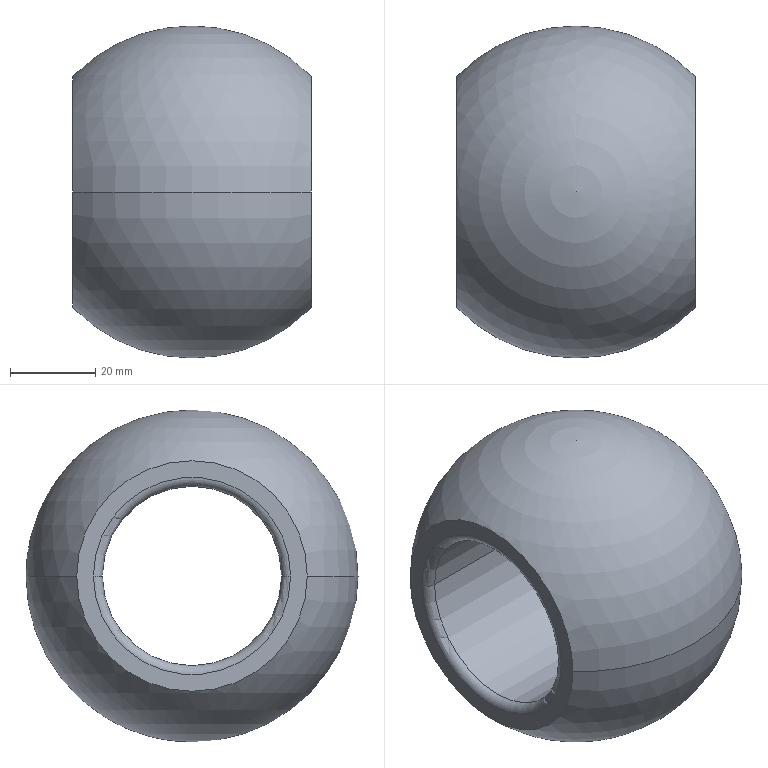Part | STEP file | Rod end bearing 1 | 1 solid | 10 faces | box 56 x 77.805 x 77.805 mm | volume 142436 mm3 | torus 4 | sphere 2 | cylinder 2 | plane 2 | commonest cylinder face diameters 42 x2
STEP:
#1=CARTESIAN_POINT('',(28.,27.007,261.));
#2=VERTEX_POINT('',#1);
#3=CARTESIAN_POINT('',(28.,-27.007,261.));
#4=VERTEX_POINT('',#3);
#5=CARTESIAN_POINT('',(28.,0.,261.));
#6=DIRECTION('',(-1.,0.,0.));
#7=DIRECTION('',(0.,-1.,0.));
#8=AXIS2_PLACEMENT_3D('',#5,#6,#7);
#9=CIRCLE('',#8,27.007);
#10=EDGE_CURVE('',#2,#4,#9,.T.);
#11=ORIENTED_EDGE('',*,*,#10,.T.);
#12=CARTESIAN_POINT('',(-28.,-27.007,261.));
#13=VERTEX_POINT('',#12);
#14=CARTESIAN_POINT('',(0.,0.,261.));
#15=DIRECTION('',(0.,0.,-1.));
#16=DIRECTION('',(0.,1.,0.));
#17=AXIS2_PLACEMENT_3D('',#14,#15,#16);
#18=CIRCLE('',#17,38.902);
#19=EDGE_CURVE('',#4,#13,#18,.T.);
#20=ORIENTED_EDGE('',*,*,#19,.T.);
#21=CARTESIAN_POINT('',(-28.,27.007,261.));
#22=VERTEX_POINT('',#21);
#23=CARTESIAN_POINT('',(-28.,0.,261.));
#24=DIRECTION('',(-1.,0.,0.));
#25=DIRECTION('',(0.,-1.,0.));
#26=AXIS2_PLACEMENT_3D('',#23,#24,#25);
#27=CIRCLE('',#26,27.007);
#28=EDGE_CURVE('',#22,#13,#27,.T.);
#29=ORIENTED_EDGE('',*,*,#28,.F.);
#30=CARTESIAN_POINT('',(0.,0.,261.));
#31=DIRECTION('',(0.,0.,1.));
#32=DIRECTION('',(1.,0.,0.));
#33=AXIS2_PLACEMENT_3D('',#30,#31,#32);
#34=CIRCLE('',#33,38.902);
#35=EDGE_CURVE('',#2,#22,#34,.T.);
#36=ORIENTED_EDGE('',*,*,#35,.F.);
#37=EDGE_LOOP('',(#11,#20,#29,#36));
#38=FACE_OUTER_BOUND('',#37,.T.);
#39=CARTESIAN_POINT('',(0.,0.,261.));
#40=DIRECTION('',(0.,0.,-1.));
#41=DIRECTION('',(0.,1.,0.));
#42=AXIS2_PLACEMENT_3D('',#39,#40,#41);
#43=SPHERICAL_SURFACE('',#42,38.902);
#44=ADVANCED_FACE('',(#38),#43,.T.);
#45=CARTESIAN_POINT('',(-28.,-23.1,261.));
#46=VERTEX_POINT('',#45);
#47=CARTESIAN_POINT('',(-28.,23.1,261.));
#48=VERTEX_POINT('',#47);
#49=CARTESIAN_POINT('',(-28.,0.,261.));
#50=DIRECTION('',(-1.,0.,0.));
#51=DIRECTION('',(0.,-1.,0.));
#52=AXIS2_PLACEMENT_3D('',#49,#50,#51);
#53=CIRCLE('',#52,23.1);
#54=EDGE_CURVE('',#46,#48,#53,.T.);
#55=ORIENTED_EDGE('',*,*,#54,.T.);
#56=CARTESIAN_POINT('',(-25.9,21.,261.));
#57=VERTEX_POINT('',#56);
#58=CARTESIAN_POINT('',(-25.9,23.1,261.));
#59=DIRECTION('',(0.,0.,1.));
#60=DIRECTION('',(0.,-1.,0.));
#61=AXIS2_PLACEMENT_3D('',#58,#59,#60);
#62=CIRCLE('',#61,2.1);
#63=EDGE_CURVE('',#48,#57,#62,.T.);
#64=ORIENTED_EDGE('',*,*,#63,.T.);
#65=CARTESIAN_POINT('',(-25.9,-21.,261.));
#66=VERTEX_POINT('',#65);
#67=CARTESIAN_POINT('',(-25.9,0.,261.));
#68=DIRECTION('',(-1.,0.,0.));
#69=DIRECTION('',(0.,-1.,0.));
#70=AXIS2_PLACEMENT_3D('',#67,#68,#69);
#71=CIRCLE('',#70,21.);
#72=EDGE_CURVE('',#66,#57,#71,.T.);
#73=ORIENTED_EDGE('',*,*,#72,.F.);
#74=CARTESIAN_POINT('',(-25.9,-23.1,261.));
#75=DIRECTION('',(0.,0.,-1.));
#76=DIRECTION('',(-1.,0.,0.));
#77=AXIS2_PLACEMENT_3D('',#74,#75,#76);
#78=CIRCLE('',#77,2.1);
#79=EDGE_CURVE('',#46,#66,#78,.T.);
#80=ORIENTED_EDGE('',*,*,#79,.F.);
#81=EDGE_LOOP('',(#55,#64,#73,#80));
#82=FACE_OUTER_BOUND('',#81,.T.);
#83=CARTESIAN_POINT('',(-25.9,0.,261.));
#84=DIRECTION('',(-1.,0.,0.));
#85=DIRECTION('',(0.,-1.,0.));
#86=AXIS2_PLACEMENT_3D('',#83,#84,#85);
#87=TOROIDAL_SURFACE('',#86,23.1,2.1);
#88=ADVANCED_FACE('',(#82),#87,.T.);
#89=CARTESIAN_POINT('',(25.9,21.,261.));
#90=VERTEX_POINT('',#89);
#91=CARTESIAN_POINT('',(25.9,-21.,261.));
#92=VERTEX_POINT('',#91);
#93=CARTESIAN_POINT('',(25.9,0.,261.));
#94=DIRECTION('',(-1.,0.,0.));
#95=DIRECTION('',(0.,-1.,0.));
#96=AXIS2_PLACEMENT_3D('',#93,#94,#95);
#97=CIRCLE('',#96,21.);
#98=EDGE_CURVE('',#90,#92,#97,.T.);
#99=ORIENTED_EDGE('',*,*,#98,.F.);
#100=CARTESIAN_POINT('',(28.,21.,261.));
#101=DIRECTION('',(-1.,0.,0.));
#102=VECTOR('',#101,1000.);
#103=LINE('',#100,#102);
#104=EDGE_CURVE('',#90,#57,#103,.T.);
#105=ORIENTED_EDGE('',*,*,#104,.T.);
#106=CARTESIAN_POINT('',(-25.9,0.,261.));
#107=DIRECTION('',(-1.,0.,0.));
#108=DIRECTION('',(0.,-1.,0.));
#109=AXIS2_PLACEMENT_3D('',#106,#107,#108);
#110=CIRCLE('',#109,21.);
#111=EDGE_CURVE('',#57,#66,#110,.T.);
#112=ORIENTED_EDGE('',*,*,#111,.T.);
#113=CARTESIAN_POINT('',(28.,-21.,261.));
#114=DIRECTION('',(-1.,0.,0.));
#115=VECTOR('',#114,1000.);
#116=LINE('',#113,#115);
#117=EDGE_CURVE('',#92,#66,#116,.T.);
#118=ORIENTED_EDGE('',*,*,#117,.F.);
#119=EDGE_LOOP('',(#99,#105,#112,#118));
#120=FACE_OUTER_BOUND('',#119,.T.);
#121=CARTESIAN_POINT('',(28.,0.,261.));
#122=DIRECTION('',(-1.,0.,0.));
#123=DIRECTION('',(0.,-1.,0.));
#124=AXIS2_PLACEMENT_3D('',#121,#122,#123);
#125=CYLINDRICAL_SURFACE('',#124,21.);
#126=ADVANCED_FACE('',(#120),#125,.F.);
#127=CARTESIAN_POINT('',(25.9,0.,261.));
#128=DIRECTION('',(-1.,0.,0.));
#129=DIRECTION('',(0.,-1.,0.));
#130=AXIS2_PLACEMENT_3D('',#127,#128,#129);
#131=CIRCLE('',#130,21.);
#132=EDGE_CURVE('',#92,#90,#131,.T.);
#133=ORIENTED_EDGE('',*,*,#132,.T.);
#134=CARTESIAN_POINT('',(28.,23.1,261.));
#135=VERTEX_POINT('',#134);
#136=CARTESIAN_POINT('',(25.9,23.1,261.));
#137=DIRECTION('',(0.,0.,1.));
#138=DIRECTION('',(0.,-1.,0.));
#139=AXIS2_PLACEMENT_3D('',#136,#137,#138);
#140=CIRCLE('',#139,2.1);
#141=EDGE_CURVE('',#90,#135,#140,.T.);
#142=ORIENTED_EDGE('',*,*,#141,.T.);
#143=CARTESIAN_POINT('',(28.,-23.1,261.));
#144=VERTEX_POINT('',#143);
#145=CARTESIAN_POINT('',(28.,0.,261.));
#146=DIRECTION('',(-1.,0.,0.));
#147=DIRECTION('',(0.,-1.,0.));
#148=AXIS2_PLACEMENT_3D('',#145,#146,#147);
#149=CIRCLE('',#148,23.1);
#150=EDGE_CURVE('',#144,#135,#149,.T.);
#151=ORIENTED_EDGE('',*,*,#150,.F.);
#152=CARTESIAN_POINT('',(25.9,-23.1,261.));
#153=DIRECTION('',(0.,0.,-1.));
#154=DIRECTION('',(-1.,0.,0.));
#155=AXIS2_PLACEMENT_3D('',#152,#153,#154);
#156=CIRCLE('',#155,2.1);
#157=EDGE_CURVE('',#92,#144,#156,.T.);
#158=ORIENTED_EDGE('',*,*,#157,.F.);
#159=EDGE_LOOP('',(#133,#142,#151,#158));
#160=FACE_OUTER_BOUND('',#159,.T.);
#161=CARTESIAN_POINT('',(25.9,0.,261.));
#162=DIRECTION('',(-1.,0.,0.));
#163=DIRECTION('',(0.,-1.,0.));
#164=AXIS2_PLACEMENT_3D('',#161,#162,#163);
#165=TOROIDAL_SURFACE('',#164,23.1,2.1);
#166=ADVANCED_FACE('',(#160),#165,.T.);
#167=ORIENTED_EDGE('',*,*,#141,.F.);
#168=ORIENTED_EDGE('',*,*,#98,.T.);
#169=ORIENTED_EDGE('',*,*,#157,.T.);
#170=CARTESIAN_POINT('',(28.,0.,261.));
#171=DIRECTION('',(-1.,0.,0.));
#172=DIRECTION('',(0.,-1.,0.));
#173=AXIS2_PLACEMENT_3D('',#170,#171,#172);
#174=CIRCLE('',#173,23.1);
#175=EDGE_CURVE('',#135,#144,#174,.T.);
#176=ORIENTED_EDGE('',*,*,#175,.F.);
#177=EDGE_LOOP('',(#167,#168,#169,#176));
#178=FACE_OUTER_BOUND('',#177,.T.);
#179=CARTESIAN_POINT('',(25.9,0.,261.));
#180=DIRECTION('',(-1.,0.,0.));
#181=DIRECTION('',(0.,-1.,0.));
#182=AXIS2_PLACEMENT_3D('',#179,#180,#181);
#183=TOROIDAL_SURFACE('',#182,23.1,2.1);
#184=ADVANCED_FACE('',(#178),#183,.T.);
#185=ORIENTED_EDGE('',*,*,#104,.F.);
#186=ORIENTED_EDGE('',*,*,#132,.F.);
#187=ORIENTED_EDGE('',*,*,#117,.T.);
#188=ORIENTED_EDGE('',*,*,#72,.T.);
#189=EDGE_LOOP('',(#185,#186,#187,#188));
#190=FACE_OUTER_BOUND('',#189,.T.);
#191=CARTESIAN_POINT('',(28.,0.,261.));
#192=DIRECTION('',(-1.,0.,0.));
#193=DIRECTION('',(0.,-1.,0.));
#194=AXIS2_PLACEMENT_3D('',#191,#192,#193);
#195=CYLINDRICAL_SURFACE('',#194,21.);
#196=ADVANCED_FACE('',(#190),#195,.F.);
#197=ORIENTED_EDGE('',*,*,#63,.F.);
#198=CARTESIAN_POINT('',(-28.,0.,261.));
#199=DIRECTION('',(-1.,0.,0.));
#200=DIRECTION('',(0.,-1.,0.));
#201=AXIS2_PLACEMENT_3D('',#198,#199,#200);
#202=CIRCLE('',#201,23.1);
#203=EDGE_CURVE('',#48,#46,#202,.T.);
#204=ORIENTED_EDGE('',*,*,#203,.T.);
#205=ORIENTED_EDGE('',*,*,#79,.T.);
#206=ORIENTED_EDGE('',*,*,#111,.F.);
#207=EDGE_LOOP('',(#197,#204,#205,#206));
#208=FACE_OUTER_BOUND('',#207,.T.);
#209=CARTESIAN_POINT('',(-25.9,0.,261.));
#210=DIRECTION('',(-1.,0.,0.));
#211=DIRECTION('',(0.,-1.,0.));
#212=AXIS2_PLACEMENT_3D('',#209,#210,#211);
#213=TOROIDAL_SURFACE('',#212,23.1,2.1);
#214=ADVANCED_FACE('',(#208),#213,.T.);
#215=ORIENTED_EDGE('',*,*,#28,.T.);
#216=CARTESIAN_POINT('',(-28.,0.,261.));
#217=DIRECTION('',(-1.,0.,0.));
#218=DIRECTION('',(0.,-1.,0.));
#219=AXIS2_PLACEMENT_3D('',#216,#217,#218);
#220=CIRCLE('',#219,27.007);
#221=EDGE_CURVE('',#13,#22,#220,.T.);
#222=ORIENTED_EDGE('',*,*,#221,.T.);
#223=EDGE_LOOP('',(#215,#222));
#224=FACE_OUTER_BOUND('',#223,.T.);
#225=ORIENTED_EDGE('',*,*,#54,.F.);
#226=ORIENTED_EDGE('',*,*,#203,.F.);
#227=EDGE_LOOP('',(#225,#226));
#228=FACE_BOUND('',#227,.T.);
#229=CARTESIAN_POINT('',(-28.,23.1,261.));
#230=DIRECTION('',(-1.,0.,0.));
#231=DIRECTION('',(0.,-1.,0.));
#232=AXIS2_PLACEMENT_3D('',#229,#230,#231);
#233=PLANE('',#232);
#234=ADVANCED_FACE('',(#224,#228),#233,.T.);
#235=ORIENTED_EDGE('',*,*,#19,.F.);
#236=CARTESIAN_POINT('',(28.,0.,261.));
#237=DIRECTION('',(-1.,0.,0.));
#238=DIRECTION('',(0.,-1.,0.));
#239=AXIS2_PLACEMENT_3D('',#236,#237,#238);
#240=CIRCLE('',#239,27.007);
#241=EDGE_CURVE('',#4,#2,#240,.T.);
#242=ORIENTED_EDGE('',*,*,#241,.T.);
#243=ORIENTED_EDGE('',*,*,#35,.T.);
#244=ORIENTED_EDGE('',*,*,#221,.F.);
#245=EDGE_LOOP('',(#235,#242,#243,#244));
#246=FACE_OUTER_BOUND('',#245,.T.);
#247=CARTESIAN_POINT('',(0.,0.,261.));
#248=DIRECTION('',(0.,0.,-1.));
#249=DIRECTION('',(0.,1.,0.));
#250=AXIS2_PLACEMENT_3D('',#247,#248,#249);
#251=SPHERICAL_SURFACE('',#250,38.902);
#252=ADVANCED_FACE('',(#246),#251,.T.);
#253=ORIENTED_EDGE('',*,*,#150,.T.);
#254=ORIENTED_EDGE('',*,*,#175,.T.);
#255=EDGE_LOOP('',(#253,#254));
#256=FACE_BOUND('',#255,.T.);
#257=ORIENTED_EDGE('',*,*,#10,.F.);
#258=ORIENTED_EDGE('',*,*,#241,.F.);
#259=EDGE_LOOP('',(#257,#258));
#260=FACE_OUTER_BOUND('',#259,.T.);
#261=CARTESIAN_POINT('',(28.,27.007,261.));
#262=DIRECTION('',(1.,0.,0.));
#263=DIRECTION('',(0.,1.,0.));
#264=AXIS2_PLACEMENT_3D('',#261,#262,#263);
#265=PLANE('',#264);
#266=ADVANCED_FACE('',(#256,#260),#265,.T.);
#267=CLOSED_SHELL('',(#44,#88,#126,#166,#184,#196,#214,#234,#252,#266));
#268=MANIFOLD_SOLID_BREP('',#267);
#269=CARTESIAN_POINT('',(0.,0.,0.));
#270=DIRECTION('',(0.,0.,1.));
#271=DIRECTION('',(1.,0.,0.));
#272=AXIS2_PLACEMENT_3D('',#269,#270,#271);
#273=(LENGTH_UNIT()NAMED_UNIT(*)SI_UNIT(.MILLI.,.METRE.));
#274=UNCERTAINTY_MEASURE_WITH_UNIT(LENGTH_MEASURE(0.00001),#273,'','');
#275=(NAMED_UNIT(*)PLANE_ANGLE_UNIT()SI_UNIT($,.RADIAN.));
#276=(NAMED_UNIT(*)SI_UNIT($,.STERADIAN.)SOLID_ANGLE_UNIT());
#277=(GEOMETRIC_REPRESENTATION_CONTEXT(3)GLOBAL_UNCERTAINTY_ASSIGNED_CONTEXT((#274))GLOBAL_UNIT_ASSIGNED_CONTEXT((#273,#275,#276))REPRESENTATION_CONTEXT('',''));
#278=ADVANCED_BREP_SHAPE_REPRESENTATION('',(#268,#272),#277);